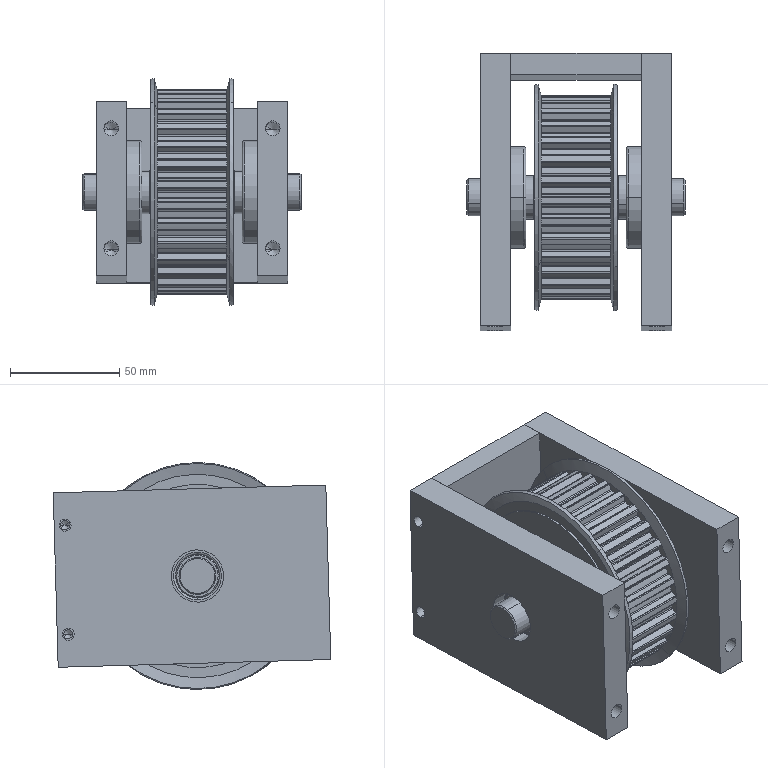Part | SolidWorks | features AEMSimFeature 1, CompositeCurve 1 | 9 solids | 693 faces | box 100 x 127.228 x 104 mm | volume 594997 mm3 | cylinder 313 | plane 178 | torus 106 | sphere 56 | cone 40 | commonest cylinder face diameters 1 x74 1.2 x70 93.65 x31 87.25 x30 20 x13 1.5 x8